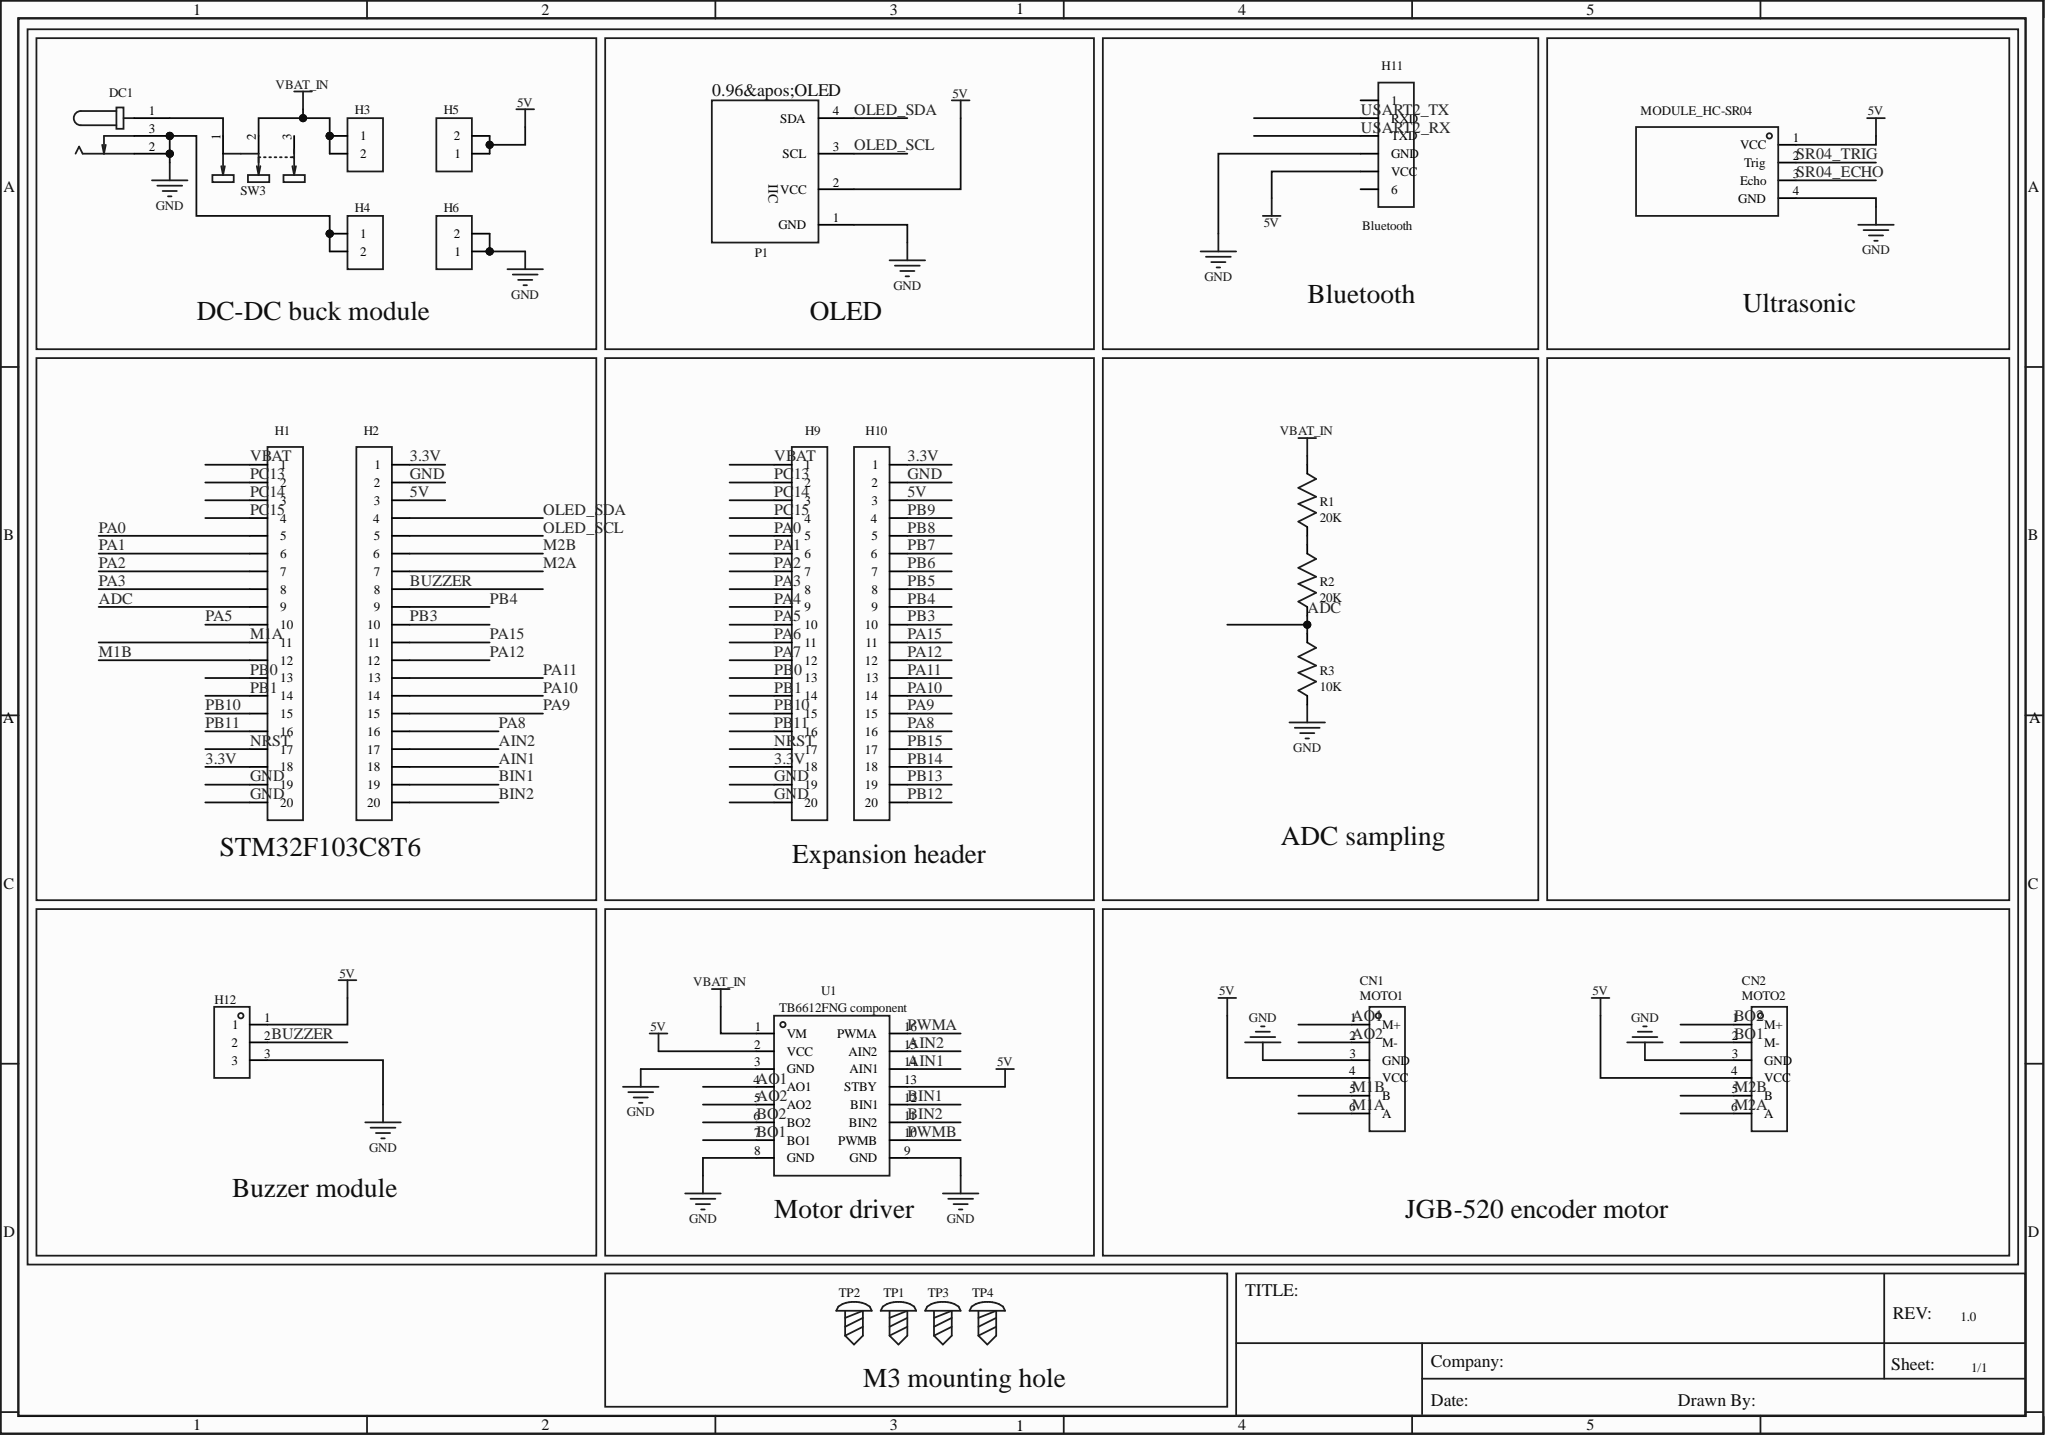Circuit board | Altium Designer | 24 parts | 44 nets
Bill of materials:
Comment,Description,Designator,Footprint,LibRef,Quantity
"MOTO1","","CN1","CONN-TH_6P-P2.50_X8821WR-06S-N2SN","X8821WR-06S-N0SN","1"
"MOTO2","","CN2","CONN-TH_6P-P2.50_X8821WR-06S-N2SN","X8821WR-06S-N0SN","1"
"DC005_C431533","","DC1","DC-IN-TH_DC005","DC005","1"
"HDR-F-2.54_1x20","","H1, H2, H9, H10","HDR-F-2.54_1X20","HDR-F-2.54_1x20","4"
"HDR-F-2.54_1x2","","H3, H4, H5, H6","HDR-F-2.54_1X2","HDR-F-2.54_1x2","4"
"Bluetooth","","H11","HDR-F-2.54_1X6","Bluetooth","1"
"","","H12","HDR-TH_3P-P2.54-V-F","HDR-F_2.54_1x3P","1"
"MODULE_HC-SR04","","NO","HC-SR04","HC-SR04","1"
"0.96OLED_4P","","P1","0.96OLED_4P","0.96'OLED-IIC(4Pin)","1"
"20K","","R1, R2","R0805","20K","2"
"10K","","R3","R0805","10K","1"
"SS-12D10L5","","SW3","SW-TH_SS-12D10L5","SS-12D10L5","1"
"M3 standoff with silkscreen","","TP1, TP2, TP3, TP4","M3铜柱","M3铜柱带丝印","4"
"TB6612FNG component","","U1","TB6612FNG封装","TB6612FNG-原件","1"
Netlist (Protel format):
[
CN1
CONN-TH_6P-P2.50_X8821WR-06S-N2SN
MOTO1



]
[
CN2
CONN-TH_6P-P2.50_X8821WR-06S-N2SN
MOTO2



]
[
DC1
DC-IN-TH_DC005
DC005_C431533



]
[
H1
HDR-F-2.54_1X20
HDR-F-2.54_1x20



]
[
H2
HDR-F-2.54_1X20
HDR-F-2.54_1x20



]
[
H3
HDR-F-2.54_1X2
HDR-F-2.54_1x2



]
[
H4
HDR-F-2.54_1X2
HDR-F-2.54_1x2



]
[
H5
HDR-F-2.54_1X2
HDR-F-2.54_1x2



]
[
H6
HDR-F-2.54_1X2
HDR-F-2.54_1x2



]
[
H9
HDR-F-2.54_1X20
HDR-F-2.54_1x20



]
[
H10
HDR-F-2.54_1X20
HDR-F-2.54_1x20



]
[
H11
HDR-F-2.54_1X6
Bluetooth



]
[
H12
HDR-TH_3P-P2.54-V-F




]
[
NO
HC-SR04
MODULE_HC-SR04



]
[
P1
0.96OLED_4P
0.96OLED_4P



]
[
R1
R0805
20K



]
[
R2
R0805
20K



]
[
R3
R0805
10K



]
[
SW3
SW-TH_SS-12D10L5
SS-12D10L5



]
[
TP1
M3铜柱
M3 standoff with silkscreen



]
[
TP2
M3铜柱
M3 standoff with silkscreen



]
[
TP3
M3铜柱
M3 standoff with silkscreen



]
[
TP4
M3铜柱
M3 standoff with silkscreen



]
[
U1
TB6612FNG封装
TB6612FNG component



]
(
VBAT_IN
H3-1
H3-2
R1-2
SW3-2
U1-1
)
(
VBAT
H1-1
H9-1
)
(
PC15
H1-4
H9-4
)
(
PC14
H1-3
H9-3
)
(
PC13
H1-2
H9-2
)
(
PB11
H1-16
H9-16
)
(
PB10
H1-15
H9-15
)
(
PB4
H2-9
H10-9
)
(
PB3
H2-10
H10-10
)
(
PB1
H1-14
H9-14
)
(
PB0
H1-13
H9-13
)
(
PA15
H2-11
H10-11
)
(
PA12
H2-12
H10-12
)
(
PA11
H2-13
H10-13
U1-16
)
(
PA10
H2-14
H10-14
)
(
PA9
H2-15
H10-15
)
(
PA8
H2-16
H10-16
U1-10
)
(
PA5
H1-10
H9-10
)
(
PA3
H1-8
H9-8
H11-3
)
(
PA2
H1-7
H9-7
H11-2
)
(
PA1
H1-6
H9-6
NO-3
)
(
PA0
H1-5
H9-5
NO-2
)
(
OLED_SDA
H2-4
H10-4
P1-4
)
(
OLED_SCL
H2-5
H10-5
P1-3
)
(
NRST
H1-17
H9-17
)
(
NetR1_1
R1-1
R2-2
)
(
NetDC1_1
DC1-1
SW3-1
)
(
M2B
CN2-5
H2-6
H10-6
)
(
M2A
CN2-6
H2-7
H10-7
)
(
M1B
CN1-5
H1-12
H9-12
)
(
M1A
CN1-6
H1-11
H9-11
)
(
GND
CN1-3
CN2-3
DC1-2
DC1-3
H1-19
H1-20
H2-2
H4-1
H4-2
H6-1
H6-2
H9-19
H9-20
H10-2
H11-4
H12-3
NO-4
P1-1
R3-1
U1-3
U1-8
U1-9
)
(
BUZZER
H2-8
H10-8
H12-2
)
(
BO2
CN2-1
U1-6
)
(
BO1
CN2-2
U1-7
)
(
BIN2
H2-20
H10-20
U1-11
)
(
BIN1
H2-19
H10-19
U1-12
)
(
AO2
CN1-2
U1-5
)
(
AO1
CN1-1
U1-4
)
(
AIN2
H2-17
H10-17
U1-15
)
(
AIN1
H2-18
H10-18
U1-14
)
(
ADC
H1-9
H9-9
R2-1
R3-2
)
(
5V
CN1-4
CN2-4
H2-3
H5-1
H5-2
H10-3
H11-5
H12-1
NO-1
P1-2
U1-2
U1-13
)
(
3.3V
H1-18
H2-1
H9-18
H10-1
)